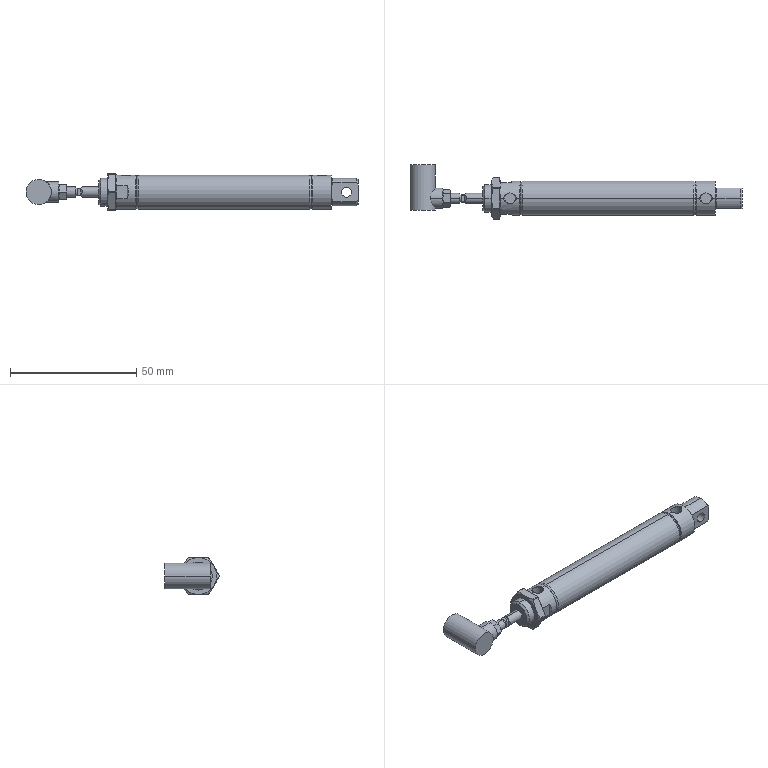Part | SolidWorks | 5 solids | 159 faces | box 131.292 x 21.537 x 14.5 mm | volume 12191 mm3 | plane 54 | cone 53 | cylinder 52 | commonest cylinder face diameters 10 x11 4 x10 13.5 x6 16.5 x6 11 x5 4.283 x4